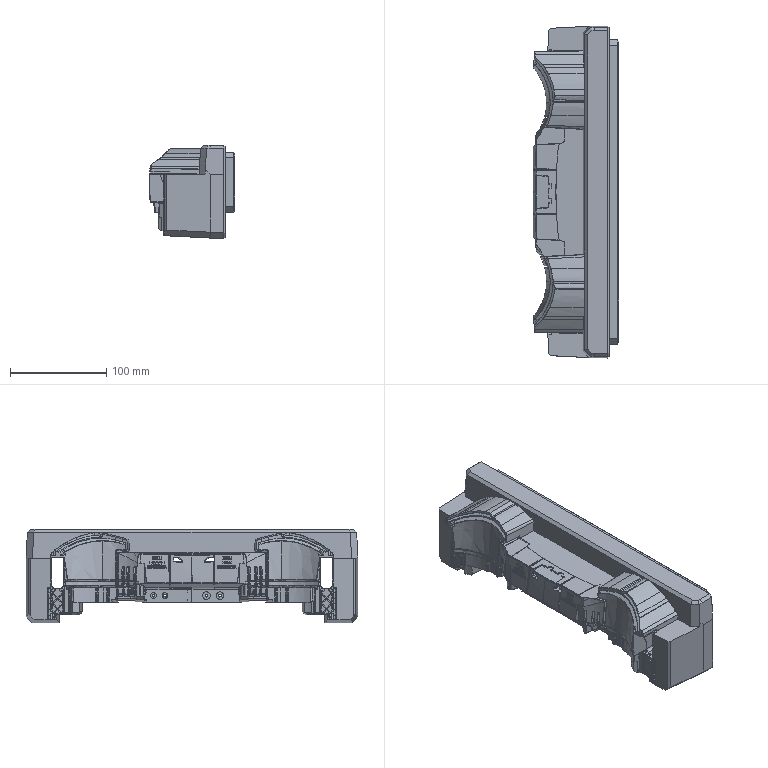Part | Creo | 2 solids | 2829 faces | box 88.793 x 345 x 97.284 mm | volume 1632945 mm3 | plane 829 | cylinder 804 | spline 539 | other 445 | sphere 161 | cone 36 | torus 15 | commonest cylinder face diameters 0.402 x346 1.005 x108 2.01 x50 1 x14 1.608 x14 15 x14